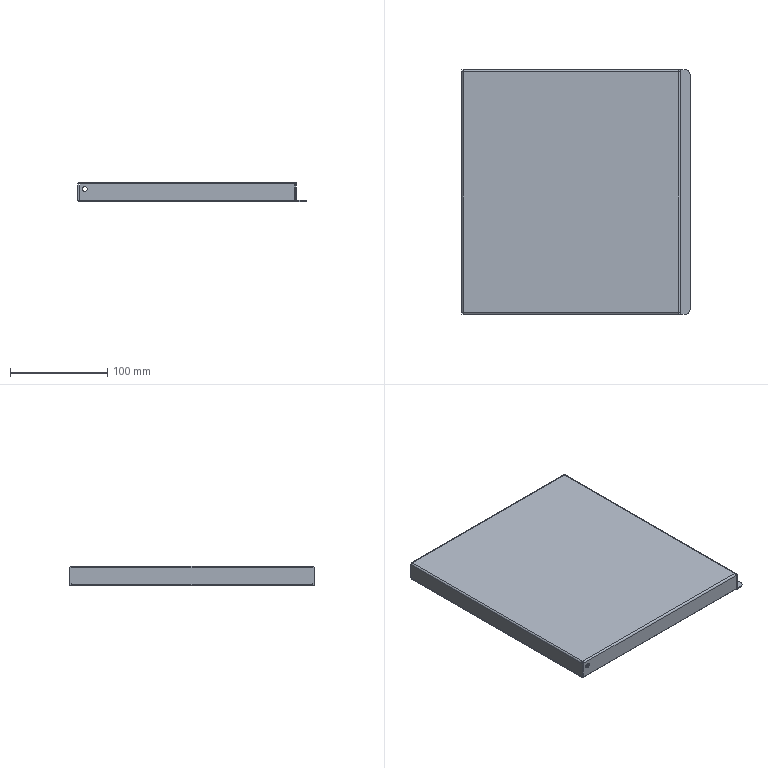Part | 1 solid | 112 faces | box 234.3 x 251 x 20 mm | volume 123828 mm3 | plane 90 | cylinder 22 | commonest cylinder face diameters 0.2 x8 3.2 x8 5.2 x4 10 x2